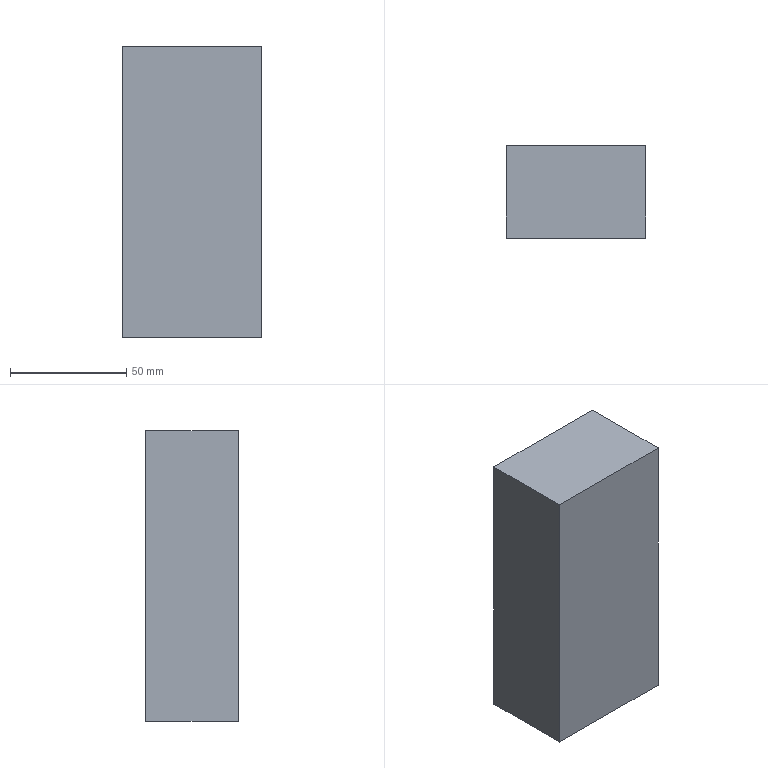Part | NX | features solid 2 | 1 solid | 6 faces | box 60 x 40 x 125 mm | volume 300000 mm3 | plane 6
STEP:
#1=CARTESIAN_POINT('',(430.,-270.,405.));
#2=VERTEX_POINT('',#1);
#3=CARTESIAN_POINT('',(430.,-310.,405.));
#4=VERTEX_POINT('',#3);
#5=CARTESIAN_POINT('',(430.,-270.,405.));
#6=DIRECTION('',(0.,1.,0.));
#7=VECTOR('',#6,1000.);
#8=LINE('',#5,#7);
#9=EDGE_CURVE('',#2,#4,#8,.F.);
#10=ORIENTED_EDGE('',*,*,#9,.F.);
#11=CARTESIAN_POINT('',(370.,-270.,405.));
#12=VERTEX_POINT('',#11);
#13=CARTESIAN_POINT('',(430.,-270.,405.));
#14=DIRECTION('',(-1.,0.,0.));
#15=VECTOR('',#14,1000.);
#16=LINE('',#13,#15);
#17=EDGE_CURVE('',#2,#12,#16,.T.);
#18=ORIENTED_EDGE('',*,*,#17,.T.);
#19=CARTESIAN_POINT('',(370.,-310.,405.));
#20=VERTEX_POINT('',#19);
#21=CARTESIAN_POINT('',(370.,-270.,405.));
#22=DIRECTION('',(0.,-1.,0.));
#23=VECTOR('',#22,1000.);
#24=LINE('',#21,#23);
#25=EDGE_CURVE('',#12,#20,#24,.T.);
#26=ORIENTED_EDGE('',*,*,#25,.T.);
#27=CARTESIAN_POINT('',(430.,-310.,405.));
#28=DIRECTION('',(-1.,0.,0.));
#29=VECTOR('',#28,1000.);
#30=LINE('',#27,#29);
#31=EDGE_CURVE('',#4,#20,#30,.T.);
#32=ORIENTED_EDGE('',*,*,#31,.F.);
#33=EDGE_LOOP('',(#10,#18,#26,#32));
#34=FACE_BOUND('',#33,.T.);
#35=CARTESIAN_POINT('',(430.,-270.,405.));
#36=DIRECTION('',(0.,0.,1.));
#37=DIRECTION('',(-1.,0.,0.));
#38=AXIS2_PLACEMENT_3D('',#35,#36,#37);
#39=PLANE('',#38);
#40=ADVANCED_FACE('',(#34),#39,.T.);
#41=ORIENTED_EDGE('',*,*,#25,.F.);
#42=CARTESIAN_POINT('',(370.,-270.,280.));
#43=VERTEX_POINT('',#42);
#44=CARTESIAN_POINT('',(370.,-270.,420.));
#45=DIRECTION('',(0.,0.,-1.));
#46=VECTOR('',#45,1000.);
#47=LINE('',#44,#46);
#48=EDGE_CURVE('',#12,#43,#47,.T.);
#49=ORIENTED_EDGE('',*,*,#48,.T.);
#50=CARTESIAN_POINT('',(370.,-310.,280.));
#51=VERTEX_POINT('',#50);
#52=CARTESIAN_POINT('',(370.,-270.,280.));
#53=DIRECTION('',(0.,1.,0.));
#54=VECTOR('',#53,1000.);
#55=LINE('',#52,#54);
#56=EDGE_CURVE('',#43,#51,#55,.F.);
#57=ORIENTED_EDGE('',*,*,#56,.T.);
#58=CARTESIAN_POINT('',(370.,-310.,420.));
#59=DIRECTION('',(0.,0.,-1.));
#60=VECTOR('',#59,1000.);
#61=LINE('',#58,#60);
#62=EDGE_CURVE('',#20,#51,#61,.T.);
#63=ORIENTED_EDGE('',*,*,#62,.F.);
#64=EDGE_LOOP('',(#41,#49,#57,#63));
#65=FACE_BOUND('',#64,.T.);
#66=CARTESIAN_POINT('',(370.,-270.,420.));
#67=DIRECTION('',(-1.,0.,0.));
#68=DIRECTION('',(0.,0.,-1.));
#69=AXIS2_PLACEMENT_3D('',#66,#67,#68);
#70=PLANE('',#69);
#71=ADVANCED_FACE('',(#65),#70,.T.);
#72=ORIENTED_EDGE('',*,*,#56,.F.);
#73=CARTESIAN_POINT('',(430.,-270.,280.));
#74=VERTEX_POINT('',#73);
#75=CARTESIAN_POINT('',(430.,-270.,280.));
#76=DIRECTION('',(1.,0.,0.));
#77=VECTOR('',#76,1000.);
#78=LINE('',#75,#77);
#79=EDGE_CURVE('',#74,#43,#78,.F.);
#80=ORIENTED_EDGE('',*,*,#79,.F.);
#81=CARTESIAN_POINT('',(430.,-310.,280.));
#82=VERTEX_POINT('',#81);
#83=CARTESIAN_POINT('',(430.,-270.,280.));
#84=DIRECTION('',(0.,-1.,0.));
#85=VECTOR('',#84,1000.);
#86=LINE('',#83,#85);
#87=EDGE_CURVE('',#74,#82,#86,.T.);
#88=ORIENTED_EDGE('',*,*,#87,.T.);
#89=CARTESIAN_POINT('',(430.,-310.,280.));
#90=DIRECTION('',(1.,0.,0.));
#91=VECTOR('',#90,1000.);
#92=LINE('',#89,#91);
#93=EDGE_CURVE('',#82,#51,#92,.F.);
#94=ORIENTED_EDGE('',*,*,#93,.T.);
#95=EDGE_LOOP('',(#72,#80,#88,#94));
#96=FACE_BOUND('',#95,.T.);
#97=CARTESIAN_POINT('',(430.,-270.,280.));
#98=DIRECTION('',(0.,0.,1.));
#99=DIRECTION('',(-1.,0.,0.));
#100=AXIS2_PLACEMENT_3D('',#97,#98,#99);
#101=PLANE('',#100);
#102=ADVANCED_FACE('',(#96),#101,.F.);
#103=ORIENTED_EDGE('',*,*,#93,.F.);
#104=CARTESIAN_POINT('',(430.,-310.,420.));
#105=DIRECTION('',(0.,0.,1.));
#106=VECTOR('',#105,1000.);
#107=LINE('',#104,#106);
#108=EDGE_CURVE('',#4,#82,#107,.F.);
#109=ORIENTED_EDGE('',*,*,#108,.F.);
#110=ORIENTED_EDGE('',*,*,#31,.T.);
#111=ORIENTED_EDGE('',*,*,#62,.T.);
#112=EDGE_LOOP('',(#103,#109,#110,#111));
#113=FACE_BOUND('',#112,.T.);
#114=CARTESIAN_POINT('',(430.,-310.,420.));
#115=DIRECTION('',(0.,-1.,0.));
#116=DIRECTION('',(0.,0.,1.));
#117=AXIS2_PLACEMENT_3D('',#114,#115,#116);
#118=PLANE('',#117);
#119=ADVANCED_FACE('',(#113),#118,.T.);
#120=CARTESIAN_POINT('',(430.,-270.,420.));
#121=DIRECTION('',(0.,0.,-1.));
#122=VECTOR('',#121,1000.);
#123=LINE('',#120,#122);
#124=EDGE_CURVE('',#2,#74,#123,.T.);
#125=ORIENTED_EDGE('',*,*,#124,.F.);
#126=ORIENTED_EDGE('',*,*,#9,.T.);
#127=ORIENTED_EDGE('',*,*,#108,.T.);
#128=ORIENTED_EDGE('',*,*,#87,.F.);
#129=EDGE_LOOP('',(#125,#126,#127,#128));
#130=FACE_BOUND('',#129,.T.);
#131=CARTESIAN_POINT('',(430.,-270.,420.));
#132=DIRECTION('',(-1.,0.,0.));
#133=DIRECTION('',(0.,0.,-1.));
#134=AXIS2_PLACEMENT_3D('',#131,#132,#133);
#135=PLANE('',#134);
#136=ADVANCED_FACE('',(#130),#135,.F.);
#137=ORIENTED_EDGE('',*,*,#79,.T.);
#138=ORIENTED_EDGE('',*,*,#48,.F.);
#139=ORIENTED_EDGE('',*,*,#17,.F.);
#140=ORIENTED_EDGE('',*,*,#124,.T.);
#141=EDGE_LOOP('',(#137,#138,#139,#140));
#142=FACE_BOUND('',#141,.T.);
#143=CARTESIAN_POINT('',(430.,-270.,420.));
#144=DIRECTION('',(0.,-1.,0.));
#145=DIRECTION('',(0.,0.,1.));
#146=AXIS2_PLACEMENT_3D('',#143,#144,#145);
#147=PLANE('',#146);
#148=ADVANCED_FACE('',(#142),#147,.F.);
#149=CLOSED_SHELL('',(#40,#71,#102,#119,#136,#148));
#150=MANIFOLD_SOLID_BREP('',#149);
#151=(LENGTH_UNIT()NAMED_UNIT(*)SI_UNIT(.MILLI.,.METRE.));
#152=UNCERTAINTY_MEASURE_WITH_UNIT(LENGTH_MEASURE(0.00001),#151,'','');
#153=(NAMED_UNIT(*)PLANE_ANGLE_UNIT()SI_UNIT($,.RADIAN.));
#154=(NAMED_UNIT(*)SI_UNIT($,.STERADIAN.)SOLID_ANGLE_UNIT());
#155=(GEOMETRIC_REPRESENTATION_CONTEXT(3)GLOBAL_UNCERTAINTY_ASSIGNED_CONTEXT((#152))GLOBAL_UNIT_ASSIGNED_CONTEXT((#151,#153,#154))REPRESENTATION_CONTEXT('',''));
#156=ADVANCED_BREP_SHAPE_REPRESENTATION('',(#150),#155);